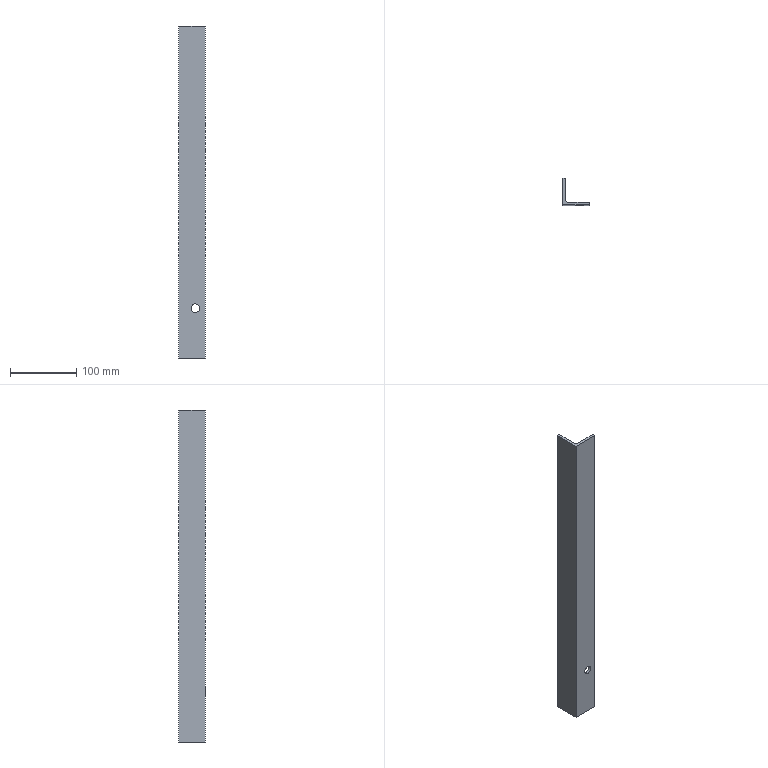Part | SolidWorks | features Extrusion 1, ICE 1 | 1 solid | 13 faces | box 40 x 40 x 500 mm | volume 153770 mm3 | plane 8 | cylinder 5 | commonest cylinder face diameters 2.667 x2 13 x2 10 x1
STEP:
#1=CARTESIAN_POINT('',(31.5,0.,75.));
#2=VERTEX_POINT('',#1);
#3=CARTESIAN_POINT('',(18.5,0.,75.));
#4=VERTEX_POINT('',#3);
#5=CARTESIAN_POINT('',(25.,0.,75.));
#6=DIRECTION('',(0.,1.,0.));
#7=DIRECTION('',(0.,0.,-1.));
#8=AXIS2_PLACEMENT_3D('',#5,#6,#7);
#9=CIRCLE('',#8,6.5);
#10=EDGE_CURVE('',#2,#4,#9,.T.);
#11=ORIENTED_EDGE('',*,*,#10,.F.);
#12=CARTESIAN_POINT('',(31.5,4.,75.));
#13=VERTEX_POINT('',#12);
#14=CARTESIAN_POINT('',(31.5,-0.001,75.));
#15=DIRECTION('',(0.,1.,0.));
#16=VECTOR('',#15,1000.);
#17=LINE('',#14,#16);
#18=EDGE_CURVE('',#2,#13,#17,.T.);
#19=ORIENTED_EDGE('',*,*,#18,.T.);
#20=CARTESIAN_POINT('',(18.5,4.,75.));
#21=VERTEX_POINT('',#20);
#22=CARTESIAN_POINT('',(25.,4.,75.));
#23=DIRECTION('',(0.,1.,0.));
#24=DIRECTION('',(-1.,0.,0.));
#25=AXIS2_PLACEMENT_3D('',#22,#23,#24);
#26=CIRCLE('',#25,6.5);
#27=EDGE_CURVE('',#13,#21,#26,.T.);
#28=ORIENTED_EDGE('',*,*,#27,.T.);
#29=CARTESIAN_POINT('',(18.5,-0.001,75.));
#30=DIRECTION('',(0.,1.,0.));
#31=VECTOR('',#30,1000.);
#32=LINE('',#29,#31);
#33=EDGE_CURVE('',#4,#21,#32,.T.);
#34=ORIENTED_EDGE('',*,*,#33,.F.);
#35=EDGE_LOOP('',(#11,#19,#28,#34));
#36=FACE_OUTER_BOUND('',#35,.T.);
#37=CARTESIAN_POINT('',(25.,-0.001,75.));
#38=DIRECTION('',(0.,1.,0.));
#39=DIRECTION('',(-1.,0.,0.));
#40=AXIS2_PLACEMENT_3D('',#37,#38,#39);
#41=CYLINDRICAL_SURFACE('',#40,6.5);
#42=ADVANCED_FACE('',(#36),#41,.F.);
#43=CARTESIAN_POINT('',(9.,4.,0.));
#44=VERTEX_POINT('',#43);
#45=CARTESIAN_POINT('',(4.,9.,0.));
#46=VERTEX_POINT('',#45);
#47=CARTESIAN_POINT('',(9.,9.,0.));
#48=DIRECTION('',(0.,0.,-1.));
#49=DIRECTION('',(-1.,0.,0.));
#50=AXIS2_PLACEMENT_3D('',#47,#48,#49);
#51=CIRCLE('',#50,5.);
#52=EDGE_CURVE('',#44,#46,#51,.T.);
#53=ORIENTED_EDGE('',*,*,#52,.T.);
#54=CARTESIAN_POINT('',(4.,9.,500.));
#55=VERTEX_POINT('',#54);
#56=CARTESIAN_POINT('',(4.,9.,500.));
#57=DIRECTION('',(0.,0.,-1.));
#58=VECTOR('',#57,1000.);
#59=LINE('',#56,#58);
#60=EDGE_CURVE('',#55,#46,#59,.T.);
#61=ORIENTED_EDGE('',*,*,#60,.F.);
#62=CARTESIAN_POINT('',(9.,4.,500.));
#63=VERTEX_POINT('',#62);
#64=CARTESIAN_POINT('',(9.,9.,500.));
#65=DIRECTION('',(0.,0.,-1.));
#66=DIRECTION('',(-1.,0.,0.));
#67=AXIS2_PLACEMENT_3D('',#64,#65,#66);
#68=CIRCLE('',#67,5.);
#69=EDGE_CURVE('',#63,#55,#68,.T.);
#70=ORIENTED_EDGE('',*,*,#69,.F.);
#71=CARTESIAN_POINT('',(9.,4.,500.));
#72=DIRECTION('',(0.,0.,-1.));
#73=VECTOR('',#72,1000.);
#74=LINE('',#71,#73);
#75=EDGE_CURVE('',#63,#44,#74,.T.);
#76=ORIENTED_EDGE('',*,*,#75,.T.);
#77=EDGE_LOOP('',(#53,#61,#70,#76));
#78=FACE_OUTER_BOUND('',#77,.T.);
#79=CARTESIAN_POINT('',(9.,9.,500.));
#80=DIRECTION('',(0.,0.,-1.));
#81=DIRECTION('',(-1.,0.,0.));
#82=AXIS2_PLACEMENT_3D('',#79,#80,#81);
#83=CYLINDRICAL_SURFACE('',#82,5.);
#84=ADVANCED_FACE('',(#78),#83,.F.);
#85=CARTESIAN_POINT('',(4.,38.667,0.));
#86=VERTEX_POINT('',#85);
#87=CARTESIAN_POINT('',(4.,38.667,0.));
#88=DIRECTION('',(0.,-1.,0.));
#89=VECTOR('',#88,1000.);
#90=LINE('',#87,#89);
#91=EDGE_CURVE('',#86,#46,#90,.T.);
#92=ORIENTED_EDGE('',*,*,#91,.F.);
#93=CARTESIAN_POINT('',(4.,38.667,500.));
#94=VERTEX_POINT('',#93);
#95=CARTESIAN_POINT('',(4.,38.667,500.));
#96=DIRECTION('',(0.,0.,-1.));
#97=VECTOR('',#96,1000.);
#98=LINE('',#95,#97);
#99=EDGE_CURVE('',#94,#86,#98,.T.);
#100=ORIENTED_EDGE('',*,*,#99,.F.);
#101=CARTESIAN_POINT('',(4.,38.667,500.));
#102=DIRECTION('',(0.,-1.,0.));
#103=VECTOR('',#102,1000.);
#104=LINE('',#101,#103);
#105=EDGE_CURVE('',#94,#55,#104,.T.);
#106=ORIENTED_EDGE('',*,*,#105,.T.);
#107=ORIENTED_EDGE('',*,*,#60,.T.);
#108=EDGE_LOOP('',(#92,#100,#106,#107));
#109=FACE_OUTER_BOUND('',#108,.T.);
#110=CARTESIAN_POINT('',(4.,38.667,500.));
#111=DIRECTION('',(1.,0.,0.));
#112=DIRECTION('',(0.,1.,0.));
#113=AXIS2_PLACEMENT_3D('',#110,#111,#112);
#114=PLANE('',#113);
#115=ADVANCED_FACE('',(#109),#114,.T.);
#116=CARTESIAN_POINT('',(2.667,40.,0.));
#117=VERTEX_POINT('',#116);
#118=CARTESIAN_POINT('',(2.667,38.667,0.));
#119=DIRECTION('',(0.,0.,-1.));
#120=DIRECTION('',(-1.,0.,0.));
#121=AXIS2_PLACEMENT_3D('',#118,#119,#120);
#122=CIRCLE('',#121,1.333);
#123=EDGE_CURVE('',#117,#86,#122,.T.);
#124=ORIENTED_EDGE('',*,*,#123,.F.);
#125=CARTESIAN_POINT('',(2.667,40.,500.));
#126=VERTEX_POINT('',#125);
#127=CARTESIAN_POINT('',(2.667,40.,500.));
#128=DIRECTION('',(0.,0.,-1.));
#129=VECTOR('',#128,1000.);
#130=LINE('',#127,#129);
#131=EDGE_CURVE('',#126,#117,#130,.T.);
#132=ORIENTED_EDGE('',*,*,#131,.F.);
#133=CARTESIAN_POINT('',(2.667,38.667,500.));
#134=DIRECTION('',(0.,0.,-1.));
#135=DIRECTION('',(-1.,0.,0.));
#136=AXIS2_PLACEMENT_3D('',#133,#134,#135);
#137=CIRCLE('',#136,1.333);
#138=EDGE_CURVE('',#126,#94,#137,.T.);
#139=ORIENTED_EDGE('',*,*,#138,.T.);
#140=ORIENTED_EDGE('',*,*,#99,.T.);
#141=EDGE_LOOP('',(#124,#132,#139,#140));
#142=FACE_OUTER_BOUND('',#141,.T.);
#143=CARTESIAN_POINT('',(2.667,38.667,500.));
#144=DIRECTION('',(0.,0.,-1.));
#145=DIRECTION('',(-1.,0.,0.));
#146=AXIS2_PLACEMENT_3D('',#143,#144,#145);
#147=CYLINDRICAL_SURFACE('',#146,1.333);
#148=ADVANCED_FACE('',(#142),#147,.T.);
#149=CARTESIAN_POINT('',(0.,40.,0.));
#150=VERTEX_POINT('',#149);
#151=CARTESIAN_POINT('',(0.,40.,0.));
#152=DIRECTION('',(1.,0.,0.));
#153=VECTOR('',#152,1000.);
#154=LINE('',#151,#153);
#155=EDGE_CURVE('',#150,#117,#154,.T.);
#156=ORIENTED_EDGE('',*,*,#155,.F.);
#157=CARTESIAN_POINT('',(0.,40.,500.));
#158=VERTEX_POINT('',#157);
#159=CARTESIAN_POINT('',(0.,40.,500.));
#160=DIRECTION('',(0.,0.,-1.));
#161=VECTOR('',#160,1000.);
#162=LINE('',#159,#161);
#163=EDGE_CURVE('',#158,#150,#162,.T.);
#164=ORIENTED_EDGE('',*,*,#163,.F.);
#165=CARTESIAN_POINT('',(0.,40.,500.));
#166=DIRECTION('',(1.,0.,0.));
#167=VECTOR('',#166,1000.);
#168=LINE('',#165,#167);
#169=EDGE_CURVE('',#158,#126,#168,.T.);
#170=ORIENTED_EDGE('',*,*,#169,.T.);
#171=ORIENTED_EDGE('',*,*,#131,.T.);
#172=EDGE_LOOP('',(#156,#164,#170,#171));
#173=FACE_OUTER_BOUND('',#172,.T.);
#174=CARTESIAN_POINT('',(0.,40.,500.));
#175=DIRECTION('',(0.,1.,0.));
#176=DIRECTION('',(0.,0.,1.));
#177=AXIS2_PLACEMENT_3D('',#174,#175,#176);
#178=PLANE('',#177);
#179=ADVANCED_FACE('',(#173),#178,.T.);
#180=CARTESIAN_POINT('',(0.,0.,0.));
#181=VERTEX_POINT('',#180);
#182=CARTESIAN_POINT('',(0.,0.,0.));
#183=DIRECTION('',(0.,1.,0.));
#184=VECTOR('',#183,1000.);
#185=LINE('',#182,#184);
#186=EDGE_CURVE('',#181,#150,#185,.T.);
#187=ORIENTED_EDGE('',*,*,#186,.F.);
#188=CARTESIAN_POINT('',(0.,0.,500.));
#189=VERTEX_POINT('',#188);
#190=CARTESIAN_POINT('',(0.,0.,500.));
#191=DIRECTION('',(0.,0.,-1.));
#192=VECTOR('',#191,1000.);
#193=LINE('',#190,#192);
#194=EDGE_CURVE('',#189,#181,#193,.T.);
#195=ORIENTED_EDGE('',*,*,#194,.F.);
#196=CARTESIAN_POINT('',(0.,0.,500.));
#197=DIRECTION('',(0.,1.,0.));
#198=VECTOR('',#197,1000.);
#199=LINE('',#196,#198);
#200=EDGE_CURVE('',#189,#158,#199,.T.);
#201=ORIENTED_EDGE('',*,*,#200,.T.);
#202=ORIENTED_EDGE('',*,*,#163,.T.);
#203=EDGE_LOOP('',(#187,#195,#201,#202));
#204=FACE_OUTER_BOUND('',#203,.T.);
#205=CARTESIAN_POINT('',(0.,0.,500.));
#206=DIRECTION('',(-1.,0.,0.));
#207=DIRECTION('',(0.,0.,1.));
#208=AXIS2_PLACEMENT_3D('',#205,#206,#207);
#209=PLANE('',#208);
#210=ADVANCED_FACE('',(#204),#209,.T.);
#211=CARTESIAN_POINT('',(25.,0.,75.));
#212=DIRECTION('',(0.,1.,0.));
#213=DIRECTION('',(0.,0.,-1.));
#214=AXIS2_PLACEMENT_3D('',#211,#212,#213);
#215=CIRCLE('',#214,6.5);
#216=EDGE_CURVE('',#4,#2,#215,.T.);
#217=ORIENTED_EDGE('',*,*,#216,.T.);
#218=ORIENTED_EDGE('',*,*,#10,.T.);
#219=EDGE_LOOP('',(#217,#218));
#220=FACE_BOUND('',#219,.T.);
#221=CARTESIAN_POINT('',(40.,0.,0.));
#222=VERTEX_POINT('',#221);
#223=CARTESIAN_POINT('',(40.,0.,0.));
#224=DIRECTION('',(-1.,0.,0.));
#225=VECTOR('',#224,1000.);
#226=LINE('',#223,#225);
#227=EDGE_CURVE('',#222,#181,#226,.T.);
#228=ORIENTED_EDGE('',*,*,#227,.F.);
#229=CARTESIAN_POINT('',(40.,0.,500.));
#230=VERTEX_POINT('',#229);
#231=CARTESIAN_POINT('',(40.,0.,500.));
#232=DIRECTION('',(0.,0.,-1.));
#233=VECTOR('',#232,1000.);
#234=LINE('',#231,#233);
#235=EDGE_CURVE('',#230,#222,#234,.T.);
#236=ORIENTED_EDGE('',*,*,#235,.F.);
#237=CARTESIAN_POINT('',(40.,0.,500.));
#238=DIRECTION('',(-1.,0.,0.));
#239=VECTOR('',#238,1000.);
#240=LINE('',#237,#239);
#241=EDGE_CURVE('',#230,#189,#240,.T.);
#242=ORIENTED_EDGE('',*,*,#241,.T.);
#243=ORIENTED_EDGE('',*,*,#194,.T.);
#244=EDGE_LOOP('',(#228,#236,#242,#243));
#245=FACE_OUTER_BOUND('',#244,.T.);
#246=CARTESIAN_POINT('',(40.,0.,500.));
#247=DIRECTION('',(0.,-1.,0.));
#248=DIRECTION('',(0.,0.,-1.));
#249=AXIS2_PLACEMENT_3D('',#246,#247,#248);
#250=PLANE('',#249);
#251=ADVANCED_FACE('',(#220,#245),#250,.T.);
#252=CARTESIAN_POINT('',(40.,2.667,0.));
#253=VERTEX_POINT('',#252);
#254=CARTESIAN_POINT('',(40.,0.,0.));
#255=DIRECTION('',(0.,1.,0.));
#256=VECTOR('',#255,1000.);
#257=LINE('',#254,#256);
#258=EDGE_CURVE('',#222,#253,#257,.T.);
#259=ORIENTED_EDGE('',*,*,#258,.T.);
#260=CARTESIAN_POINT('',(40.,2.667,500.));
#261=VERTEX_POINT('',#260);
#262=CARTESIAN_POINT('',(40.,2.667,500.));
#263=DIRECTION('',(0.,0.,-1.));
#264=VECTOR('',#263,1000.);
#265=LINE('',#262,#264);
#266=EDGE_CURVE('',#261,#253,#265,.T.);
#267=ORIENTED_EDGE('',*,*,#266,.F.);
#268=CARTESIAN_POINT('',(40.,0.,500.));
#269=DIRECTION('',(0.,1.,0.));
#270=VECTOR('',#269,1000.);
#271=LINE('',#268,#270);
#272=EDGE_CURVE('',#230,#261,#271,.T.);
#273=ORIENTED_EDGE('',*,*,#272,.F.);
#274=ORIENTED_EDGE('',*,*,#235,.T.);
#275=EDGE_LOOP('',(#259,#267,#273,#274));
#276=FACE_OUTER_BOUND('',#275,.T.);
#277=CARTESIAN_POINT('',(40.,0.,500.));
#278=DIRECTION('',(-1.,0.,0.));
#279=DIRECTION('',(0.,-1.,0.));
#280=AXIS2_PLACEMENT_3D('',#277,#278,#279);
#281=PLANE('',#280);
#282=ADVANCED_FACE('',(#276),#281,.F.);
#283=CARTESIAN_POINT('',(38.667,4.,0.));
#284=VERTEX_POINT('',#283);
#285=CARTESIAN_POINT('',(38.667,2.667,0.));
#286=DIRECTION('',(0.,0.,1.));
#287=DIRECTION('',(1.,0.,0.));
#288=AXIS2_PLACEMENT_3D('',#285,#286,#287);
#289=CIRCLE('',#288,1.333);
#290=EDGE_CURVE('',#253,#284,#289,.T.);
#291=ORIENTED_EDGE('',*,*,#290,.T.);
#292=CARTESIAN_POINT('',(38.667,4.,500.));
#293=VERTEX_POINT('',#292);
#294=CARTESIAN_POINT('',(38.667,4.,500.));
#295=DIRECTION('',(0.,0.,-1.));
#296=VECTOR('',#295,1000.);
#297=LINE('',#294,#296);
#298=EDGE_CURVE('',#293,#284,#297,.T.);
#299=ORIENTED_EDGE('',*,*,#298,.F.);
#300=CARTESIAN_POINT('',(38.667,2.667,500.));
#301=DIRECTION('',(0.,0.,1.));
#302=DIRECTION('',(1.,0.,0.));
#303=AXIS2_PLACEMENT_3D('',#300,#301,#302);
#304=CIRCLE('',#303,1.333);
#305=EDGE_CURVE('',#261,#293,#304,.T.);
#306=ORIENTED_EDGE('',*,*,#305,.F.);
#307=ORIENTED_EDGE('',*,*,#266,.T.);
#308=EDGE_LOOP('',(#291,#299,#306,#307));
#309=FACE_OUTER_BOUND('',#308,.T.);
#310=CARTESIAN_POINT('',(38.667,2.667,500.));
#311=DIRECTION('',(0.,0.,-1.));
#312=DIRECTION('',(-1.,0.,0.));
#313=AXIS2_PLACEMENT_3D('',#310,#311,#312);
#314=CYLINDRICAL_SURFACE('',#313,1.333);
#315=ADVANCED_FACE('',(#309),#314,.T.);
#316=CARTESIAN_POINT('',(25.,4.,75.));
#317=DIRECTION('',(0.,1.,0.));
#318=DIRECTION('',(-1.,0.,0.));
#319=AXIS2_PLACEMENT_3D('',#316,#317,#318);
#320=CIRCLE('',#319,6.5);
#321=EDGE_CURVE('',#21,#13,#320,.T.);
#322=ORIENTED_EDGE('',*,*,#321,.F.);
#323=ORIENTED_EDGE('',*,*,#27,.F.);
#324=EDGE_LOOP('',(#322,#323));
#325=FACE_BOUND('',#324,.T.);
#326=CARTESIAN_POINT('',(9.,4.,0.));
#327=DIRECTION('',(1.,0.,0.));
#328=VECTOR('',#327,1000.);
#329=LINE('',#326,#328);
#330=EDGE_CURVE('',#44,#284,#329,.T.);
#331=ORIENTED_EDGE('',*,*,#330,.F.);
#332=ORIENTED_EDGE('',*,*,#75,.F.);
#333=CARTESIAN_POINT('',(9.,4.,500.));
#334=DIRECTION('',(1.,0.,0.));
#335=VECTOR('',#334,1000.);
#336=LINE('',#333,#335);
#337=EDGE_CURVE('',#63,#293,#336,.T.);
#338=ORIENTED_EDGE('',*,*,#337,.T.);
#339=ORIENTED_EDGE('',*,*,#298,.T.);
#340=EDGE_LOOP('',(#331,#332,#338,#339));
#341=FACE_OUTER_BOUND('',#340,.T.);
#342=CARTESIAN_POINT('',(9.,4.,500.));
#343=DIRECTION('',(0.,1.,0.));
#344=DIRECTION('',(-1.,0.,0.));
#345=AXIS2_PLACEMENT_3D('',#342,#343,#344);
#346=PLANE('',#345);
#347=ADVANCED_FACE('',(#325,#341),#346,.T.);
#348=ORIENTED_EDGE('',*,*,#69,.T.);
#349=ORIENTED_EDGE('',*,*,#105,.F.);
#350=ORIENTED_EDGE('',*,*,#138,.F.);
#351=ORIENTED_EDGE('',*,*,#169,.F.);
#352=ORIENTED_EDGE('',*,*,#200,.F.);
#353=ORIENTED_EDGE('',*,*,#241,.F.);
#354=ORIENTED_EDGE('',*,*,#272,.T.);
#355=ORIENTED_EDGE('',*,*,#305,.T.);
#356=ORIENTED_EDGE('',*,*,#337,.F.);
#357=EDGE_LOOP('',(#348,#349,#350,#351,#352,#353,#354,#355,#356));
#358=FACE_OUTER_BOUND('',#357,.T.);
#359=CARTESIAN_POINT('',(9.,9.,500.));
#360=DIRECTION('',(0.,0.,-1.));
#361=DIRECTION('',(-1.,0.,0.));
#362=AXIS2_PLACEMENT_3D('',#359,#360,#361);
#363=PLANE('',#362);
#364=ADVANCED_FACE('',(#358),#363,.F.);
#365=ORIENTED_EDGE('',*,*,#52,.F.);
#366=ORIENTED_EDGE('',*,*,#330,.T.);
#367=ORIENTED_EDGE('',*,*,#290,.F.);
#368=ORIENTED_EDGE('',*,*,#258,.F.);
#369=ORIENTED_EDGE('',*,*,#227,.T.);
#370=ORIENTED_EDGE('',*,*,#186,.T.);
#371=ORIENTED_EDGE('',*,*,#155,.T.);
#372=ORIENTED_EDGE('',*,*,#123,.T.);
#373=ORIENTED_EDGE('',*,*,#91,.T.);
#374=EDGE_LOOP('',(#365,#366,#367,#368,#369,#370,#371,#372,#373));
#375=FACE_OUTER_BOUND('',#374,.T.);
#376=CARTESIAN_POINT('',(9.,9.,0.));
#377=DIRECTION('',(0.,0.,-1.));
#378=DIRECTION('',(-1.,0.,0.));
#379=AXIS2_PLACEMENT_3D('',#376,#377,#378);
#380=PLANE('',#379);
#381=ADVANCED_FACE('',(#375),#380,.T.);
#382=ORIENTED_EDGE('',*,*,#18,.F.);
#383=ORIENTED_EDGE('',*,*,#216,.F.);
#384=ORIENTED_EDGE('',*,*,#33,.T.);
#385=ORIENTED_EDGE('',*,*,#321,.T.);
#386=EDGE_LOOP('',(#382,#383,#384,#385));
#387=FACE_OUTER_BOUND('',#386,.T.);
#388=CARTESIAN_POINT('',(25.,-0.001,75.));
#389=DIRECTION('',(0.,1.,0.));
#390=DIRECTION('',(-1.,0.,0.));
#391=AXIS2_PLACEMENT_3D('',#388,#389,#390);
#392=CYLINDRICAL_SURFACE('',#391,6.5);
#393=ADVANCED_FACE('',(#387),#392,.F.);
#394=CLOSED_SHELL('',(#42,#84,#115,#148,#179,#210,#251,#282,#315,#347,#364,#381,#393));
#395=MANIFOLD_SOLID_BREP('',#394);
#396=CARTESIAN_POINT('',(0.,0.,0.));
#397=DIRECTION('',(0.,0.,1.));
#398=DIRECTION('',(1.,0.,0.));
#399=AXIS2_PLACEMENT_3D('',#396,#397,#398);
#400=(LENGTH_UNIT()NAMED_UNIT(*)SI_UNIT(.MILLI.,.METRE.));
#401=UNCERTAINTY_MEASURE_WITH_UNIT(LENGTH_MEASURE(0.00001),#400,'','');
#402=(NAMED_UNIT(*)PLANE_ANGLE_UNIT()SI_UNIT($,.RADIAN.));
#403=(NAMED_UNIT(*)SI_UNIT($,.STERADIAN.)SOLID_ANGLE_UNIT());
#404=(GEOMETRIC_REPRESENTATION_CONTEXT(3)GLOBAL_UNCERTAINTY_ASSIGNED_CONTEXT((#401))GLOBAL_UNIT_ASSIGNED_CONTEXT((#400,#402,#403))REPRESENTATION_CONTEXT('',''));
#405=ADVANCED_BREP_SHAPE_REPRESENTATION('',(#395,#399),#404);